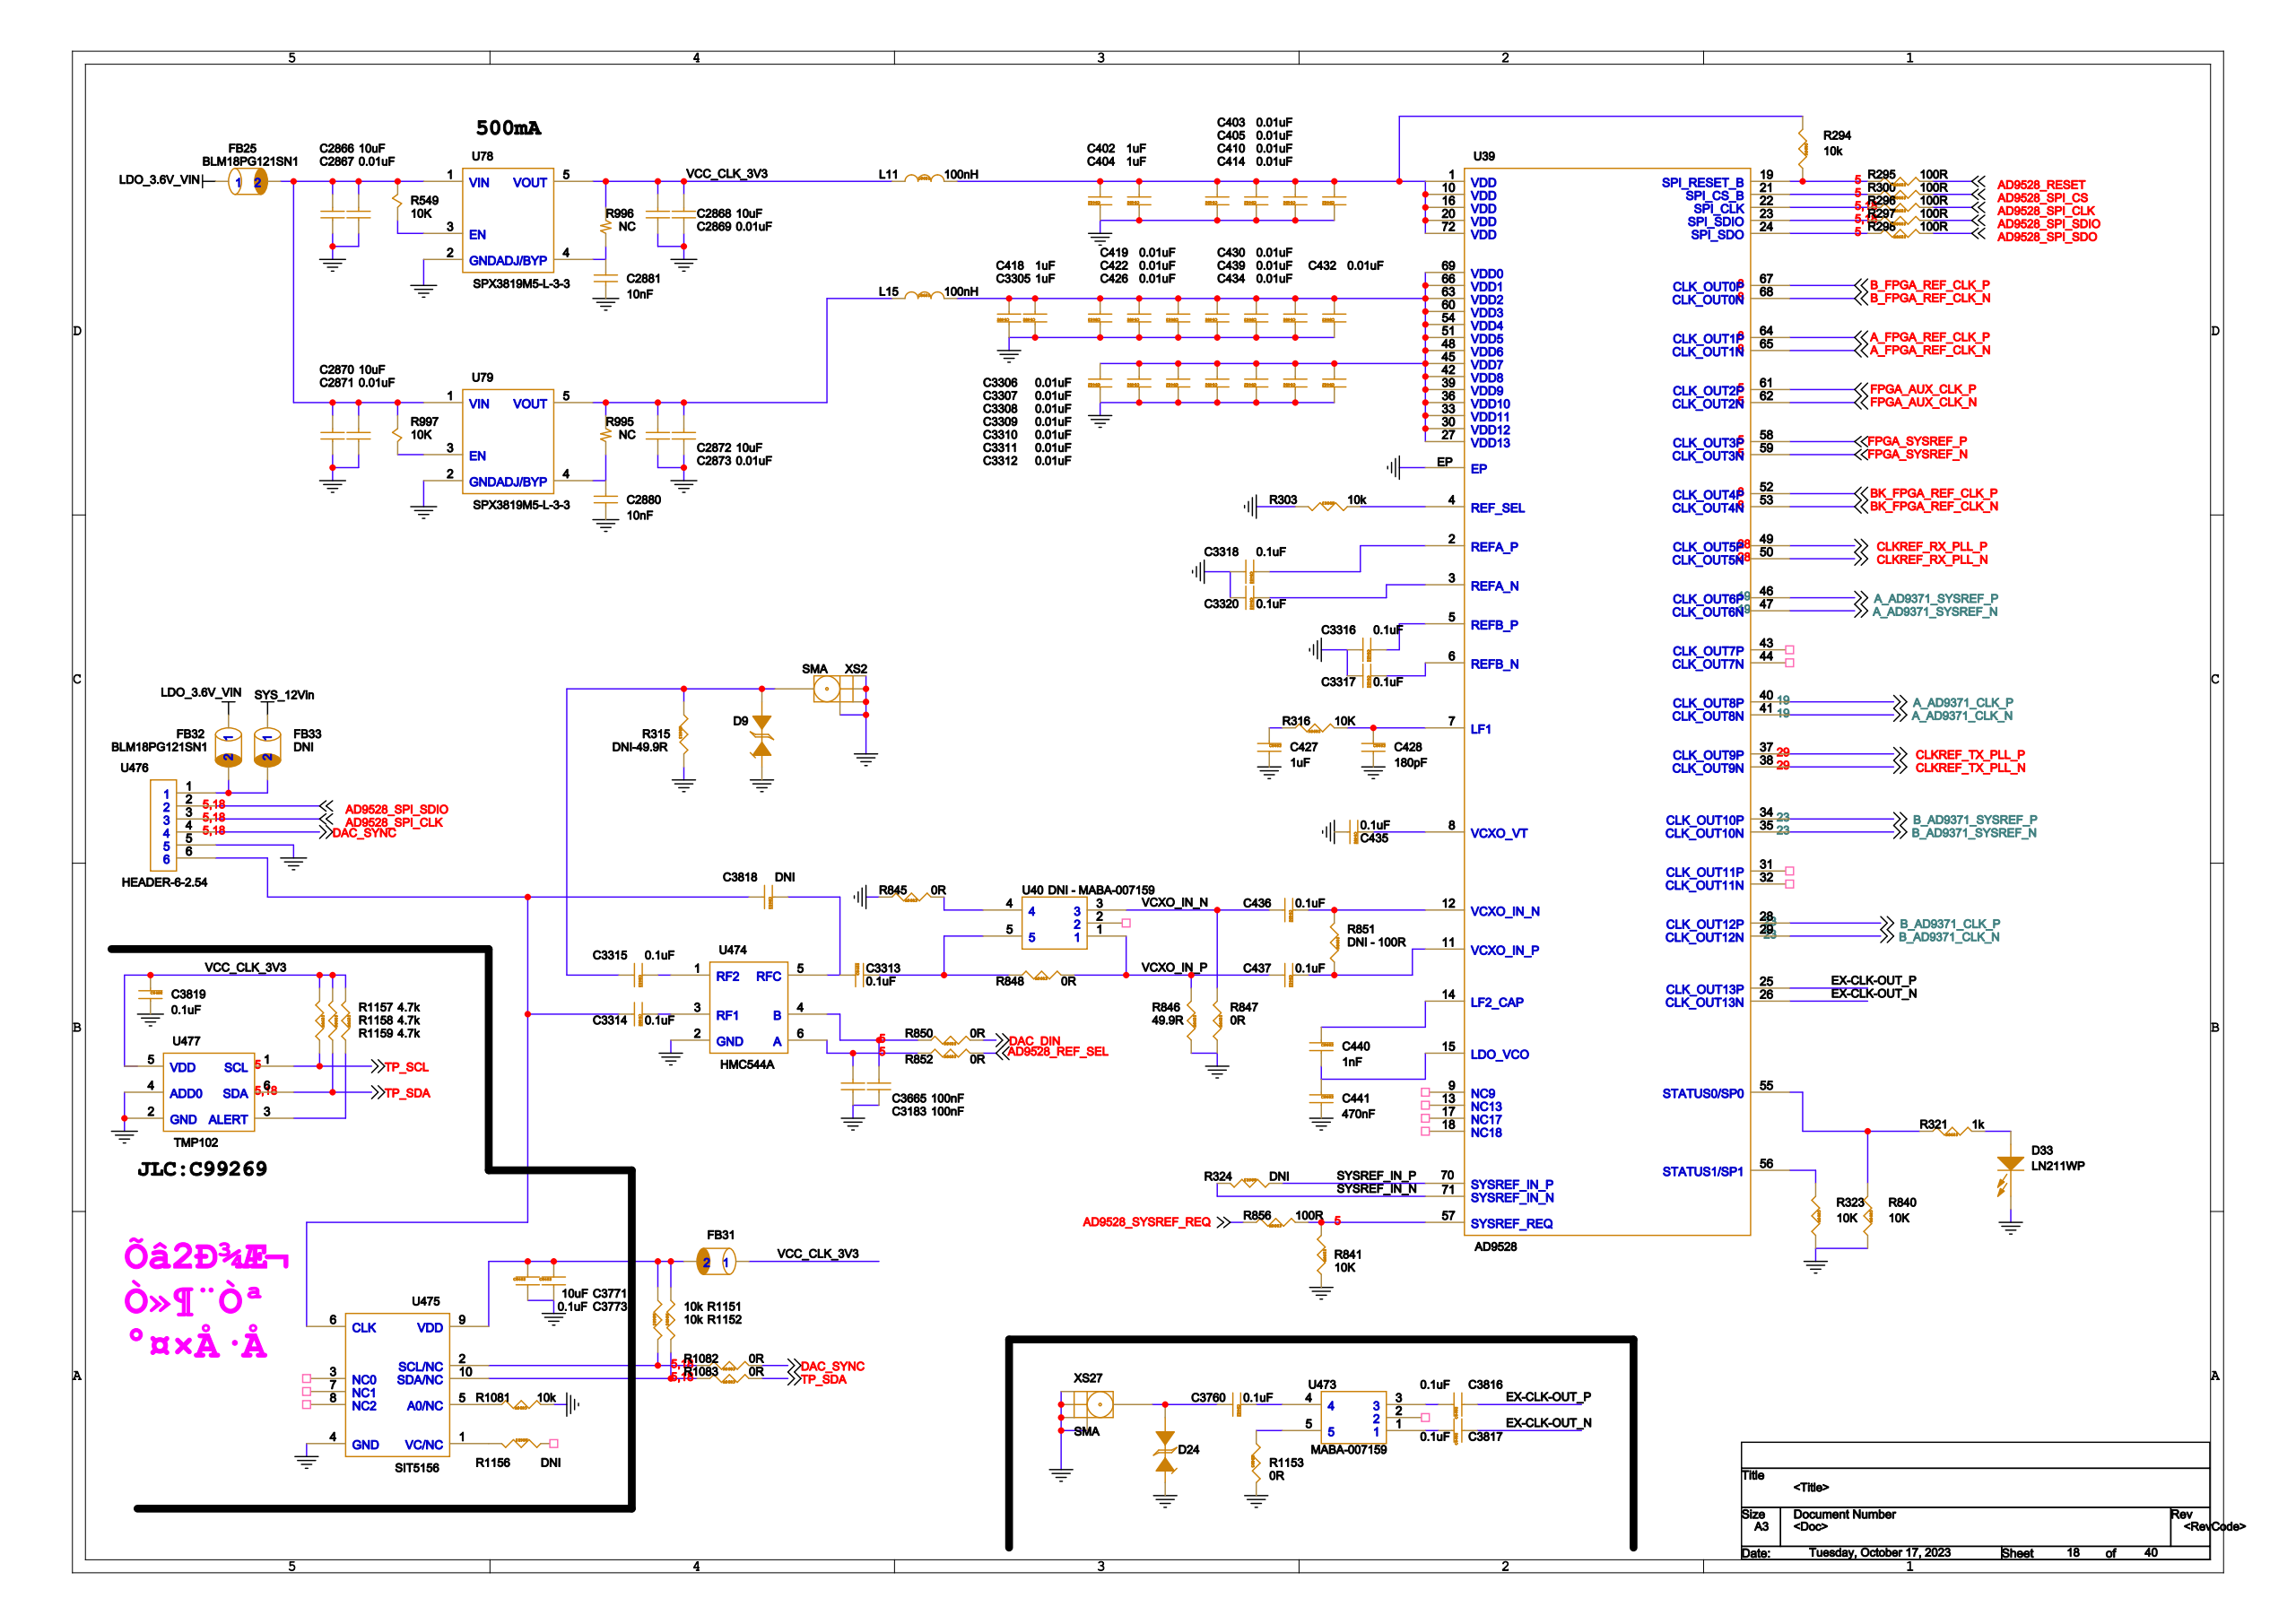Circuit board | Cadence Allegro | 1793 parts | 1223 nets | one sheet of the schematic
Parts on this sheet (reference | value | footprint):
C402 | 1uF | C0402
C403 | 0.01uF | C0402
C404 | 1uF | C0402
C405 | 0.01uF | C0402
C410 | 0.01uF | C0402
C414 | 0.01uF | C0402
C418 | 1uF | C0402
C419 | 0.01uF | C0402
C422 | 0.01uF | C0402
C426 | 0.01uF | C0402
C427 | 1uF | C0402
C428 | 180pF | C0402
C430 | 0.01uF | C0402
C432 | 0.01uF | C0402
C434 | 0.01uF | C0402
C435 | 0.1uF | C0402
C436 | 0.1uF | C0402
C437 | 0.1uF | C0402
C439 | 0.01uF | C0402
C440 | 1nF | C0402
C441 | 470nF | C0402
C2866 | 10uF | C0402
C2867 | 0.01uF | C0402
C2868 | 10uF | C0402
C2869 | 0.01uF | C0402
C2870 | 10uF | C0402
C2871 | 0.01uF | C0402
C2872 | 10uF | C0402
C2873 | 0.01uF | C0402
C2880 | 10nF | C0402
C2881 | 10nF | C0402
C3183 | 100nF | C0402
C3305 | 1uF | C0402
C3306 | 0.01uF | C0402
C3307 | 0.01uF | C0402
C3308 | 0.01uF | C0402
C3309 | 0.01uF | C0402
C3310 | 0.01uF | C0402
C3311 | 0.01uF | C0402
C3312 | 0.01uF | C0402
C3313 | 0.1uF | C0402
C3314 | 0.1uF | C0402
C3315 | 0.1uF | C0402
C3316 | 0.1uF | C0402
C3317 | 0.1uF | C0402
C3318 | 0.1uF | C0402
C3320 | 0.1uF | C0402
C3665 | 100nF | C0402
C3760 | 0.1uF | C0402
C3771 | 10uF | C0402
C3773 | 0.1uF | C0402
C3816 | 0.1uF | C0402
C3817 | 0.1uF | C0402
C3818 | DNI | C0402
C3819 | 0.1uF | C0402
D33 | LN211WP | D0603
FB25 | BLM18PG121SN1 | FB0603
FB31 | BLM18PG121SN1 | FB0603
FB32 | BLM18PG121SN1 | FB0603
FB33 | DNI | FB0603
L11 | 100nH | L0603
L15 | 100nH | L0603
R294 | 10k | R0402
R295 | 100R | R0402
R296 | 100R | R0402
R297 | 100R | R0402
R298 | 100R | R0402
R300 | 100R | R0402
R303 | 10k | R0402
R315 | DNI-49.9R | R0402
R316 | 10k | R0402
R321 | 1k | R0402
R323 | 10k | R0402
R324 | DNI | R0402
R549 | 10K | R0402
R840 | 10k | R0402
R841 | 10k | R0402
R845 | 0R | R0603
R846 | 49.9R | R0402
R847 | 0R | R0402
R848 | 0R | R0402
R850 | 0R | R0603
R851 | DNI - 100R | R0402
R852 | 0R | R0402
R856 | 100R | R0402
R995 | NC | R0402
R996 | NC | R0402
R997 | 10K | R0402
R1081 | 10k | R0603
R1082 | 0R | R0603
R1083 | 0R | R0603
R1151 | 10k | R0603
R1152 | 10k | R0603
R1153 | 0R | R0603
R1156 | DNI | R0402
R1157 | 4.7k | R0603
R1158 | 4.7k | R0603
R1159 | 4.7k | R0603
U39 | AD9528 | QFN72_10X10_PAD5_3X5_3
U40 | DNI - MABA-007159 | TCM1-1
U78 | SPX3819M5-L-3-3 | SOT-23-5
U79 | SPX3819M5-L-3-3 | SOT-23-5
U473 | MABA-007159 | TCM1-1
U474 | HMC544A | SOT23_6
U475 | SIT5156 | OSC-SMD_10P-L5-W3_2
U476 | HEADER-6-2.54 | DIP1X6
U477 | TMP102 | OT-563_L1_6-W1_2-P0_50-LS1_61
XS2 | SMA | SMA_5X5MM
XS27 | SMA | SMA_5X5MM
Nets of these parts (net: part-pin ...):
N699253: R321-1 R840-2 U39-55
N699257: D33-1 R321-2
GND: C402-1 C403-1 C404-1 C405-1 C410-1 C414-1 C418-1 C419-1 C422-1 C426-1 C427-2 C428-2 C430-1 C432-1 C434-1 C435-2 C439-1 C441-2 C2866-1 C2867-1 C2868-1 C2869-1 C2870-1 C2871-1 C2872-1 C2873-1 C2880-2 C2881-2 C3183-1 C3305-1 C3306-1 C3307-1 C3308-1 C3309-1 C3310-1 C3311-1 C3312-1 C3316-2 C3317-2 C3318-2 C3320-2 C3665-1 C3771-2 C3773-2 C3819-2 D33-2 R303-2 R315-1 R323-1 R840-1 R841-1 R845-1 R846-1 R847-1 R1081-2 R1153-1 U78-2 U79-2 U474-2 U475-4 U476-5 U477-2 U477-4 XS2-2 XS2-3 XS2-4 XS2-5 XS27-2 XS27-3 XS27-4 XS27-5 U39-EP
TP_SCL: R1157-1 U477-1
VCC_CLK_3V3: C2868-2 C2869-2 C3819-1 FB31-1 L11-1 R996-1 R1157-2 R1158-2 R1159-2 U78-5 U477-5
TP_SDA: R1083-2 R1158-1 U477-6
N18762557: R1159-1 U477-3
N18608325: C3760-2 XS27-1
N16884353: C3315-2 R315-2 XS2-1
SYS_12VIN: FB33-1
LDO_3.6V_VIN: FB25-1 FB32-1
N696673: R294-1 R295-1 U39-19
N16863185: C402-2 C403-2 C404-2 C405-2 C410-2 C414-2 L11-2 R294-2 U39-1 U39-10 U39-16 U39-20 U39-72
N18294913: R303-1 U39-4
N698575: C427-1 R316-1
N698579: C428-1 R316-2 U39-7
N699309: R323-2 U39-56
N16866799: R841-2 R856-2 U39-57
N18610125: C3817-1 U473-1
N18610107: C3816-1 U473-3
N18611130: C3760-1 U473-4
N18611127: R1153-2 U473-5
N18684054: C3665-2 R852-1 U474-6
N18684061: C3183-2 R850-1 U474-4
N18680886: C3314-1 U474-3
N18680889: C3315-1 U474-1
N18680784: C3313-1 C3818-1 U474-5
N186828104: R1081-1 U475-5
N18683538: C3314-2 C3818-2 U475-6 U476-6
N18682829: R1082-1 R1152-2 U475-2
N18682827: R1083-1 R1151-2 U475-10
N186828100: R1156-2 U475-1
N18682744: C3771-1 C3773-1 FB31-2 R1151-1 R1152-1 U475-9
N18685734: FB32-2 FB33-2 U476-1
AD9528_SPI_SDIO: R297-2 U476-2
AD9528_SPI_CLK: R296-2 U476-3
DAC_SYNC: R1082-2 U476-4
N16347306: C2866-2 C2867-2 C2870-2 C2871-2 FB25-2 R549-2 R997-2 U78-1 U79-1
N16347620: C2872-2 C2873-2 L15-1 R995-1 U79-5
N16885361: C3313-2 R848-1 U40-5
VCXO_IN_P: C437-2 R846-2 R848-2 U40-1
AD9528_REF_SEL: R852-2
VCXO_IN_N: C436-2 R847-2 U40-3
SYSREF_IN_P: R324-1 U39-70
SYSREF_IN_N: R324-2 U39-71
N699091: C437-1 R851-1 U39-11
N18295454: C436-1 R851-2 U39-12
CLKREF_RX_PLL_P: U39-49
CLKREF_RX_PLL_N: U39-50
CLKREF_TX_PLL_P: U39-37
CLKREF_TX_PLL_N: U39-38
N16885354: R845-2 U40-4
N16347752: C2880-1 R995-2 U79-4
N16347478: C2881-1 R996-2 U78-4
EX-CLK-OUT_P: C3816-2 U39-25
EX-CLK-OUT_N: C3817-2 U39-26
N18296686: C435-1 U39-8
N18662983: C3316-1 U39-5
N18662995: C3317-1 U39-6
N18662965: C3318-1 U39-2
N18662974: C3320-1 U39-3
A_AD9371_CLK_P: U39-40
A_AD9371_CLK_N: U39-41
A_FPGA_REF_CLK_P: U39-64
A_FPGA_REF_CLK_N: U39-65
B_FPGA_REF_CLK_P: U39-67
B_FPGA_REF_CLK_N: U39-68
B_AD9371_CLK_N: U39-29
B_AD9371_CLK_P: U39-28
N16863284: C418-2 C419-2 C422-2 C426-2 C430-2 C432-2 C434-2 C439-2 C3305-2 C3306-2 C3307-2 C3308-2 C3309-2 C3310-2 C3311-2 C3312-2 L15-2 U39-27 U39-30 U39-33 U39-36 U39-39 U39-42 U39-45 U39-48 U39-51 U39-54 U39-60 U39-63 U39-66 U39-69
B_AD9371_SYSREF_P: U39-34
B_AD9371_SYSREF_N: U39-35
A_AD9371_SYSREF_P: U39-46
A_AD9371_SYSREF_N: U39-47
N699175: C440-1 U39-14
N16417494: C440-2 C441-1 U39-15
N18280467: R549-1 U78-3
N16347748: R997-1 U79-3
AD9528_RESET: R295-2
N1528693: R296-1 U39-22
N1528729: R297-1 U39-23
N696829: R298-1 U39-24
AD9528_SPI_SDO: R298-2
N1528653: R300-1 U39-21
AD9528_SPI_CS: R300-2
AD9528_SYSREF_REQ: R856-1
DAC_DIN: R850-2
FPGA_AUX_CLK_N: U39-62
FPGA_AUX_CLK_P: U39-61
FPGA_SYSREF_N: U39-59
FPGA_SYSREF_P: U39-58
BK_FPGA_REF_CLK_N: U39-53
BK_FPGA_REF_CLK_P: U39-52